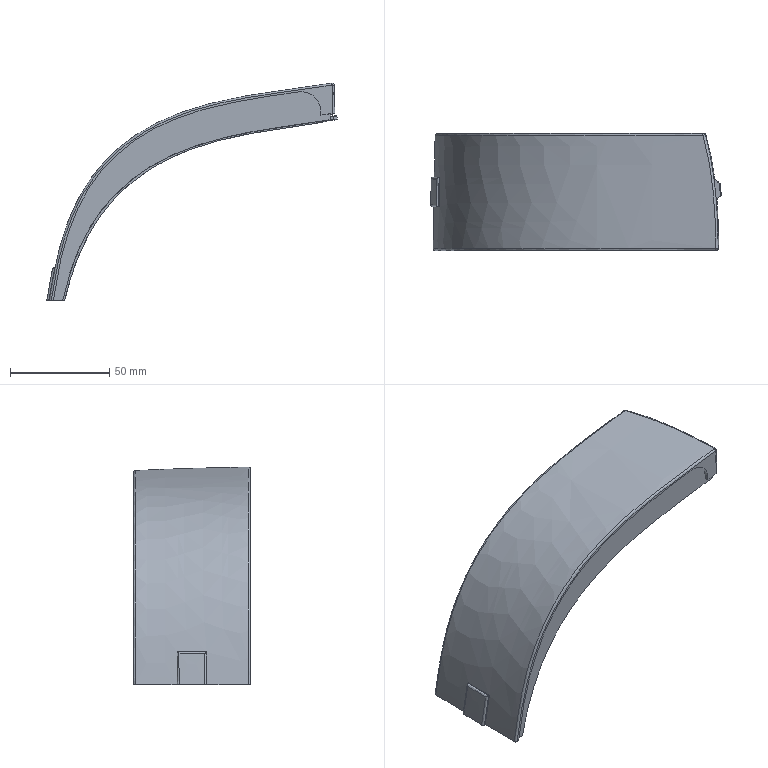Part | NX | features Body 2 | 1 solid | 79 faces | box 146.551 x 59 x 110.019 mm | volume 28651 mm3 | spline 42 | plane 25 | cylinder 6 | sphere 6 | commonest cylinder face diameters 2 x2 20 x2 399.911 x1 22072 x1